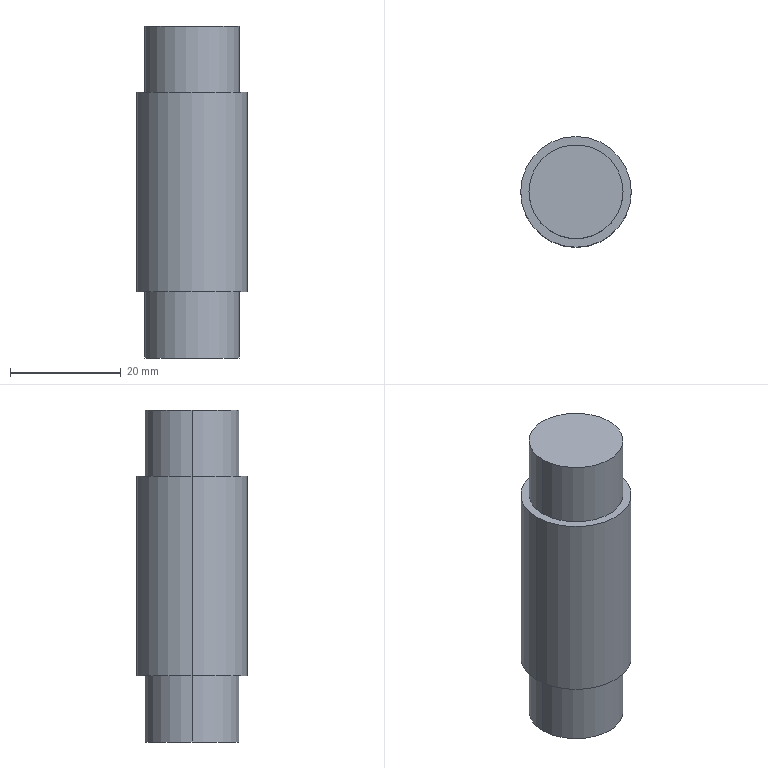Part | SolidWorks | features Extrusion 1, ICE 1, MirrorPattern 1 | 1 solid | 10 faces | box 20 x 20 x 60 mm | volume 16757 mm3 | cylinder 6 | plane 4 | commonest cylinder face diameters 17 x4 20 x2
STEP:
#1=CARTESIAN_POINT('',(8.5,0.,-30.));
#2=VERTEX_POINT('',#1);
#3=CARTESIAN_POINT('',(-8.5,0.,-30.));
#4=VERTEX_POINT('',#3);
#5=CARTESIAN_POINT('',(0.,0.,-30.));
#6=DIRECTION('',(0.,0.,1.));
#7=DIRECTION('',(1.,0.,0.));
#8=AXIS2_PLACEMENT_3D('',#5,#6,#7);
#9=CIRCLE('',#8,8.5);
#10=EDGE_CURVE('',#2,#4,#9,.T.);
#11=ORIENTED_EDGE('',*,*,#10,.T.);
#12=CARTESIAN_POINT('',(-8.5,0.,-18.));
#13=VERTEX_POINT('',#12);
#14=CARTESIAN_POINT('',(-8.5,0.,-30.));
#15=DIRECTION('',(0.,0.,1.));
#16=VECTOR('',#15,1000.);
#17=LINE('',#14,#16);
#18=EDGE_CURVE('',#4,#13,#17,.T.);
#19=ORIENTED_EDGE('',*,*,#18,.T.);
#20=CARTESIAN_POINT('',(8.5,0.,-18.));
#21=VERTEX_POINT('',#20);
#22=CARTESIAN_POINT('',(0.,0.,-18.));
#23=DIRECTION('',(0.,0.,1.));
#24=DIRECTION('',(1.,0.,0.));
#25=AXIS2_PLACEMENT_3D('',#22,#23,#24);
#26=CIRCLE('',#25,8.5);
#27=EDGE_CURVE('',#21,#13,#26,.T.);
#28=ORIENTED_EDGE('',*,*,#27,.F.);
#29=CARTESIAN_POINT('',(8.5,0.,-30.));
#30=DIRECTION('',(0.,0.,1.));
#31=VECTOR('',#30,1000.);
#32=LINE('',#29,#31);
#33=EDGE_CURVE('',#2,#21,#32,.T.);
#34=ORIENTED_EDGE('',*,*,#33,.F.);
#35=EDGE_LOOP('',(#11,#19,#28,#34));
#36=FACE_OUTER_BOUND('',#35,.T.);
#37=CARTESIAN_POINT('',(0.,0.,-30.));
#38=DIRECTION('',(0.,0.,1.));
#39=DIRECTION('',(1.,0.,0.));
#40=AXIS2_PLACEMENT_3D('',#37,#38,#39);
#41=CYLINDRICAL_SURFACE('',#40,8.5);
#42=ADVANCED_FACE('',(#36),#41,.T.);
#43=CARTESIAN_POINT('',(8.5,0.,30.));
#44=VERTEX_POINT('',#43);
#45=CARTESIAN_POINT('',(-8.5,0.,30.));
#46=VERTEX_POINT('',#45);
#47=CARTESIAN_POINT('',(0.,0.,30.));
#48=DIRECTION('',(0.,0.,1.));
#49=DIRECTION('',(1.,0.,0.));
#50=AXIS2_PLACEMENT_3D('',#47,#48,#49);
#51=CIRCLE('',#50,8.5);
#52=EDGE_CURVE('',#44,#46,#51,.T.);
#53=ORIENTED_EDGE('',*,*,#52,.F.);
#54=CARTESIAN_POINT('',(8.5,0.,18.));
#55=VERTEX_POINT('',#54);
#56=CARTESIAN_POINT('',(8.5,0.,30.));
#57=DIRECTION('',(0.,0.,-1.));
#58=VECTOR('',#57,1000.);
#59=LINE('',#56,#58);
#60=EDGE_CURVE('',#44,#55,#59,.T.);
#61=ORIENTED_EDGE('',*,*,#60,.T.);
#62=CARTESIAN_POINT('',(-8.5,0.,18.));
#63=VERTEX_POINT('',#62);
#64=CARTESIAN_POINT('',(0.,0.,18.));
#65=DIRECTION('',(0.,0.,1.));
#66=DIRECTION('',(1.,0.,0.));
#67=AXIS2_PLACEMENT_3D('',#64,#65,#66);
#68=CIRCLE('',#67,8.5);
#69=EDGE_CURVE('',#55,#63,#68,.T.);
#70=ORIENTED_EDGE('',*,*,#69,.T.);
#71=CARTESIAN_POINT('',(-8.5,0.,30.));
#72=DIRECTION('',(0.,0.,-1.));
#73=VECTOR('',#72,1000.);
#74=LINE('',#71,#73);
#75=EDGE_CURVE('',#46,#63,#74,.T.);
#76=ORIENTED_EDGE('',*,*,#75,.F.);
#77=EDGE_LOOP('',(#53,#61,#70,#76));
#78=FACE_OUTER_BOUND('',#77,.T.);
#79=CARTESIAN_POINT('',(0.,0.,30.));
#80=DIRECTION('',(0.,0.,-1.));
#81=DIRECTION('',(-1.,0.,0.));
#82=AXIS2_PLACEMENT_3D('',#79,#80,#81);
#83=CYLINDRICAL_SURFACE('',#82,8.5);
#84=ADVANCED_FACE('',(#78),#83,.T.);
#85=CARTESIAN_POINT('',(10.,0.,18.));
#86=VERTEX_POINT('',#85);
#87=CARTESIAN_POINT('',(-10.,0.,18.));
#88=VERTEX_POINT('',#87);
#89=CARTESIAN_POINT('',(0.,0.,18.));
#90=DIRECTION('',(0.,0.,1.));
#91=DIRECTION('',(1.,0.,0.));
#92=AXIS2_PLACEMENT_3D('',#89,#90,#91);
#93=CIRCLE('',#92,10.);
#94=EDGE_CURVE('',#86,#88,#93,.T.);
#95=ORIENTED_EDGE('',*,*,#94,.F.);
#96=CARTESIAN_POINT('',(10.,0.,-18.));
#97=VERTEX_POINT('',#96);
#98=CARTESIAN_POINT('',(10.,0.,18.));
#99=DIRECTION('',(0.,0.,-1.));
#100=VECTOR('',#99,1000.);
#101=LINE('',#98,#100);
#102=EDGE_CURVE('',#86,#97,#101,.T.);
#103=ORIENTED_EDGE('',*,*,#102,.T.);
#104=CARTESIAN_POINT('',(-10.,0.,-18.));
#105=VERTEX_POINT('',#104);
#106=CARTESIAN_POINT('',(0.,0.,-18.));
#107=DIRECTION('',(0.,0.,1.));
#108=DIRECTION('',(1.,0.,0.));
#109=AXIS2_PLACEMENT_3D('',#106,#107,#108);
#110=CIRCLE('',#109,10.);
#111=EDGE_CURVE('',#97,#105,#110,.T.);
#112=ORIENTED_EDGE('',*,*,#111,.T.);
#113=CARTESIAN_POINT('',(-10.,0.,18.));
#114=DIRECTION('',(0.,0.,-1.));
#115=VECTOR('',#114,1000.);
#116=LINE('',#113,#115);
#117=EDGE_CURVE('',#88,#105,#116,.T.);
#118=ORIENTED_EDGE('',*,*,#117,.F.);
#119=EDGE_LOOP('',(#95,#103,#112,#118));
#120=FACE_OUTER_BOUND('',#119,.T.);
#121=CARTESIAN_POINT('',(0.,0.,18.));
#122=DIRECTION('',(0.,0.,-1.));
#123=DIRECTION('',(-1.,0.,0.));
#124=AXIS2_PLACEMENT_3D('',#121,#122,#123);
#125=CYLINDRICAL_SURFACE('',#124,10.);
#126=ADVANCED_FACE('',(#120),#125,.T.);
#127=ORIENTED_EDGE('',*,*,#102,.F.);
#128=CARTESIAN_POINT('',(0.,0.,18.));
#129=DIRECTION('',(0.,0.,1.));
#130=DIRECTION('',(1.,0.,0.));
#131=AXIS2_PLACEMENT_3D('',#128,#129,#130);
#132=CIRCLE('',#131,10.);
#133=EDGE_CURVE('',#88,#86,#132,.T.);
#134=ORIENTED_EDGE('',*,*,#133,.F.);
#135=ORIENTED_EDGE('',*,*,#117,.T.);
#136=CARTESIAN_POINT('',(0.,0.,-18.));
#137=DIRECTION('',(0.,0.,1.));
#138=DIRECTION('',(1.,0.,0.));
#139=AXIS2_PLACEMENT_3D('',#136,#137,#138);
#140=CIRCLE('',#139,10.);
#141=EDGE_CURVE('',#105,#97,#140,.T.);
#142=ORIENTED_EDGE('',*,*,#141,.T.);
#143=EDGE_LOOP('',(#127,#134,#135,#142));
#144=FACE_OUTER_BOUND('',#143,.T.);
#145=CARTESIAN_POINT('',(0.,0.,18.));
#146=DIRECTION('',(0.,0.,-1.));
#147=DIRECTION('',(-1.,0.,0.));
#148=AXIS2_PLACEMENT_3D('',#145,#146,#147);
#149=CYLINDRICAL_SURFACE('',#148,10.);
#150=ADVANCED_FACE('',(#144),#149,.T.);
#151=CARTESIAN_POINT('',(0.,0.,18.));
#152=DIRECTION('',(0.,0.,1.));
#153=DIRECTION('',(1.,0.,0.));
#154=AXIS2_PLACEMENT_3D('',#151,#152,#153);
#155=CIRCLE('',#154,8.5);
#156=EDGE_CURVE('',#63,#55,#155,.T.);
#157=ORIENTED_EDGE('',*,*,#156,.F.);
#158=ORIENTED_EDGE('',*,*,#69,.F.);
#159=EDGE_LOOP('',(#157,#158));
#160=FACE_BOUND('',#159,.T.);
#161=ORIENTED_EDGE('',*,*,#133,.T.);
#162=ORIENTED_EDGE('',*,*,#94,.T.);
#163=EDGE_LOOP('',(#161,#162));
#164=FACE_OUTER_BOUND('',#163,.T.);
#165=CARTESIAN_POINT('',(0.,0.,18.));
#166=DIRECTION('',(0.,0.,1.));
#167=DIRECTION('',(1.,0.,0.));
#168=AXIS2_PLACEMENT_3D('',#165,#166,#167);
#169=PLANE('',#168);
#170=ADVANCED_FACE('',(#160,#164),#169,.T.);
#171=ORIENTED_EDGE('',*,*,#27,.T.);
#172=CARTESIAN_POINT('',(0.,0.,-18.));
#173=DIRECTION('',(0.,0.,1.));
#174=DIRECTION('',(1.,0.,0.));
#175=AXIS2_PLACEMENT_3D('',#172,#173,#174);
#176=CIRCLE('',#175,8.5);
#177=EDGE_CURVE('',#13,#21,#176,.T.);
#178=ORIENTED_EDGE('',*,*,#177,.T.);
#179=EDGE_LOOP('',(#171,#178));
#180=FACE_BOUND('',#179,.T.);
#181=ORIENTED_EDGE('',*,*,#141,.F.);
#182=ORIENTED_EDGE('',*,*,#111,.F.);
#183=EDGE_LOOP('',(#181,#182));
#184=FACE_OUTER_BOUND('',#183,.T.);
#185=CARTESIAN_POINT('',(0.,0.,-18.));
#186=DIRECTION('',(0.,0.,1.));
#187=DIRECTION('',(1.,0.,0.));
#188=AXIS2_PLACEMENT_3D('',#185,#186,#187);
#189=PLANE('',#188);
#190=ADVANCED_FACE('',(#180,#184),#189,.F.);
#191=ORIENTED_EDGE('',*,*,#60,.F.);
#192=CARTESIAN_POINT('',(0.,0.,30.));
#193=DIRECTION('',(0.,0.,1.));
#194=DIRECTION('',(1.,0.,0.));
#195=AXIS2_PLACEMENT_3D('',#192,#193,#194);
#196=CIRCLE('',#195,8.5);
#197=EDGE_CURVE('',#46,#44,#196,.T.);
#198=ORIENTED_EDGE('',*,*,#197,.F.);
#199=ORIENTED_EDGE('',*,*,#75,.T.);
#200=ORIENTED_EDGE('',*,*,#156,.T.);
#201=EDGE_LOOP('',(#191,#198,#199,#200));
#202=FACE_OUTER_BOUND('',#201,.T.);
#203=CARTESIAN_POINT('',(0.,0.,30.));
#204=DIRECTION('',(0.,0.,-1.));
#205=DIRECTION('',(-1.,0.,0.));
#206=AXIS2_PLACEMENT_3D('',#203,#204,#205);
#207=CYLINDRICAL_SURFACE('',#206,8.5);
#208=ADVANCED_FACE('',(#202),#207,.T.);
#209=ORIENTED_EDGE('',*,*,#197,.T.);
#210=ORIENTED_EDGE('',*,*,#52,.T.);
#211=EDGE_LOOP('',(#209,#210));
#212=FACE_OUTER_BOUND('',#211,.T.);
#213=CARTESIAN_POINT('',(0.,0.,30.));
#214=DIRECTION('',(0.,0.,1.));
#215=DIRECTION('',(1.,0.,0.));
#216=AXIS2_PLACEMENT_3D('',#213,#214,#215);
#217=PLANE('',#216);
#218=ADVANCED_FACE('',(#212),#217,.T.);
#219=ORIENTED_EDGE('',*,*,#18,.F.);
#220=CARTESIAN_POINT('',(0.,0.,-30.));
#221=DIRECTION('',(0.,0.,1.));
#222=DIRECTION('',(1.,0.,0.));
#223=AXIS2_PLACEMENT_3D('',#220,#221,#222);
#224=CIRCLE('',#223,8.5);
#225=EDGE_CURVE('',#4,#2,#224,.T.);
#226=ORIENTED_EDGE('',*,*,#225,.T.);
#227=ORIENTED_EDGE('',*,*,#33,.T.);
#228=ORIENTED_EDGE('',*,*,#177,.F.);
#229=EDGE_LOOP('',(#219,#226,#227,#228));
#230=FACE_OUTER_BOUND('',#229,.T.);
#231=CARTESIAN_POINT('',(0.,0.,-30.));
#232=DIRECTION('',(0.,0.,1.));
#233=DIRECTION('',(1.,0.,0.));
#234=AXIS2_PLACEMENT_3D('',#231,#232,#233);
#235=CYLINDRICAL_SURFACE('',#234,8.5);
#236=ADVANCED_FACE('',(#230),#235,.T.);
#237=ORIENTED_EDGE('',*,*,#10,.F.);
#238=ORIENTED_EDGE('',*,*,#225,.F.);
#239=EDGE_LOOP('',(#237,#238));
#240=FACE_OUTER_BOUND('',#239,.T.);
#241=CARTESIAN_POINT('',(0.,0.,-30.));
#242=DIRECTION('',(0.,0.,-1.));
#243=DIRECTION('',(1.,0.,0.));
#244=AXIS2_PLACEMENT_3D('',#241,#242,#243);
#245=PLANE('',#244);
#246=ADVANCED_FACE('',(#240),#245,.T.);
#247=CLOSED_SHELL('',(#42,#84,#126,#150,#170,#190,#208,#218,#236,#246));
#248=MANIFOLD_SOLID_BREP('',#247);
#249=CARTESIAN_POINT('',(0.,0.,0.));
#250=DIRECTION('',(0.,0.,1.));
#251=DIRECTION('',(1.,0.,0.));
#252=AXIS2_PLACEMENT_3D('',#249,#250,#251);
#253=(LENGTH_UNIT()NAMED_UNIT(*)SI_UNIT(.MILLI.,.METRE.));
#254=UNCERTAINTY_MEASURE_WITH_UNIT(LENGTH_MEASURE(0.00001),#253,'','');
#255=(NAMED_UNIT(*)PLANE_ANGLE_UNIT()SI_UNIT($,.RADIAN.));
#256=(NAMED_UNIT(*)SI_UNIT($,.STERADIAN.)SOLID_ANGLE_UNIT());
#257=(GEOMETRIC_REPRESENTATION_CONTEXT(3)GLOBAL_UNCERTAINTY_ASSIGNED_CONTEXT((#254))GLOBAL_UNIT_ASSIGNED_CONTEXT((#253,#255,#256))REPRESENTATION_CONTEXT('',''));
#258=ADVANCED_BREP_SHAPE_REPRESENTATION('',(#248,#252),#257);